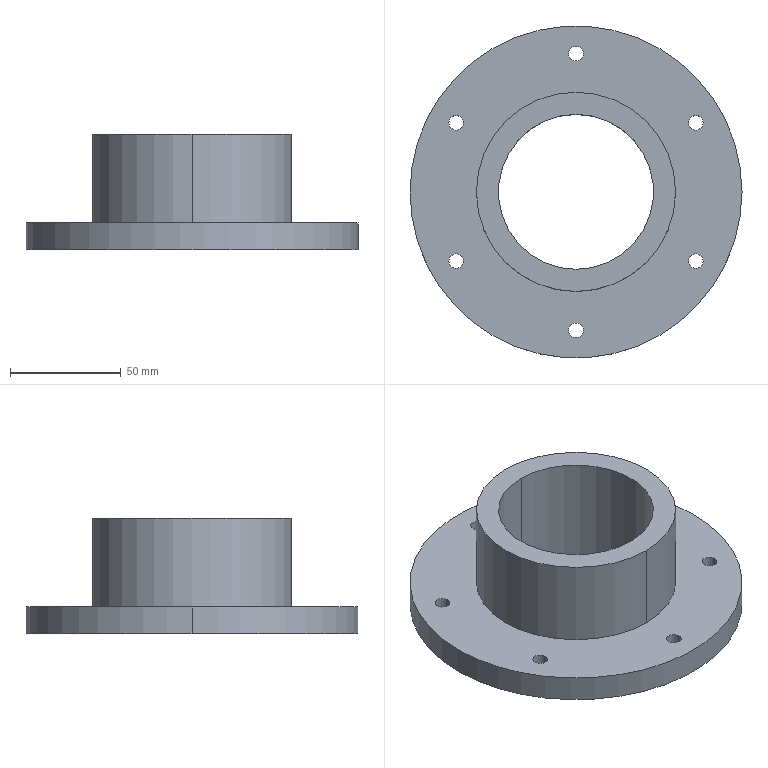Part | SolidWorks | features BaseBody 1 | 1 solid | 39 faces | box 150 x 150 x 52 mm | volume 261462 mm3 | cylinder 30 | plane 9 | commonest cylinder face diameters 6.6 x12 11 x12 70 x2 90 x2 150 x2
STEP:
#1=CARTESIAN_POINT('',(-54.127,36.75,6.8));
#2=VERTEX_POINT('',#1);
#3=CARTESIAN_POINT('',(-54.127,25.75,6.8));
#4=VERTEX_POINT('',#3);
#5=CARTESIAN_POINT('',(-54.127,31.25,6.8));
#6=DIRECTION('',(0.,0.,1.));
#7=DIRECTION('',(0.,1.,0.));
#8=AXIS2_PLACEMENT_3D('',#5,#6,#7);
#9=CIRCLE('',#8,5.5);
#10=EDGE_CURVE('',#2,#4,#9,.T.);
#11=ORIENTED_EDGE('',*,*,#10,.T.);
#12=CARTESIAN_POINT('',(-54.127,25.75,0.));
#13=VERTEX_POINT('',#12);
#14=CARTESIAN_POINT('',(-54.127,25.75,6.8));
#15=DIRECTION('',(0.,0.,-1.));
#16=VECTOR('',#15,1000.);
#17=LINE('',#14,#16);
#18=EDGE_CURVE('',#4,#13,#17,.T.);
#19=ORIENTED_EDGE('',*,*,#18,.T.);
#20=CARTESIAN_POINT('',(-54.127,36.75,0.));
#21=VERTEX_POINT('',#20);
#22=CARTESIAN_POINT('',(-54.127,31.25,0.));
#23=DIRECTION('',(0.,0.,-1.));
#24=DIRECTION('',(0.,1.,0.));
#25=AXIS2_PLACEMENT_3D('',#22,#23,#24);
#26=CIRCLE('',#25,5.5);
#27=EDGE_CURVE('',#13,#21,#26,.T.);
#28=ORIENTED_EDGE('',*,*,#27,.T.);
#29=CARTESIAN_POINT('',(-54.127,36.75,6.8));
#30=DIRECTION('',(0.,0.,-1.));
#31=VECTOR('',#30,1000.);
#32=LINE('',#29,#31);
#33=EDGE_CURVE('',#2,#21,#32,.T.);
#34=ORIENTED_EDGE('',*,*,#33,.F.);
#35=EDGE_LOOP('',(#11,#19,#28,#34));
#36=FACE_OUTER_BOUND('',#35,.T.);
#37=CARTESIAN_POINT('',(-54.127,31.25,6.8));
#38=DIRECTION('',(0.,0.,-1.));
#39=DIRECTION('',(0.,1.,0.));
#40=AXIS2_PLACEMENT_3D('',#37,#38,#39);
#41=CYLINDRICAL_SURFACE('',#40,5.5);
#42=ADVANCED_FACE('',(#36),#41,.F.);
#43=CARTESIAN_POINT('',(0.,35.,52.));
#44=VERTEX_POINT('',#43);
#45=CARTESIAN_POINT('',(0.,-35.,52.));
#46=VERTEX_POINT('',#45);
#47=CARTESIAN_POINT('',(0.,0.,52.));
#48=DIRECTION('',(0.,0.,1.));
#49=DIRECTION('',(0.,1.,0.));
#50=AXIS2_PLACEMENT_3D('',#47,#48,#49);
#51=CIRCLE('',#50,35.);
#52=EDGE_CURVE('',#44,#46,#51,.T.);
#53=ORIENTED_EDGE('',*,*,#52,.T.);
#54=CARTESIAN_POINT('',(0.,-35.,0.));
#55=VERTEX_POINT('',#54);
#56=CARTESIAN_POINT('',(0.,-35.,52.));
#57=DIRECTION('',(0.,0.,-1.));
#58=VECTOR('',#57,1000.);
#59=LINE('',#56,#58);
#60=EDGE_CURVE('',#46,#55,#59,.T.);
#61=ORIENTED_EDGE('',*,*,#60,.T.);
#62=CARTESIAN_POINT('',(0.,35.,0.));
#63=VERTEX_POINT('',#62);
#64=CARTESIAN_POINT('',(0.,0.,0.));
#65=DIRECTION('',(0.,0.,-1.));
#66=DIRECTION('',(0.,1.,0.));
#67=AXIS2_PLACEMENT_3D('',#64,#65,#66);
#68=CIRCLE('',#67,35.);
#69=EDGE_CURVE('',#55,#63,#68,.T.);
#70=ORIENTED_EDGE('',*,*,#69,.T.);
#71=CARTESIAN_POINT('',(0.,35.,52.));
#72=DIRECTION('',(0.,0.,-1.));
#73=VECTOR('',#72,1000.);
#74=LINE('',#71,#73);
#75=EDGE_CURVE('',#44,#63,#74,.T.);
#76=ORIENTED_EDGE('',*,*,#75,.F.);
#77=EDGE_LOOP('',(#53,#61,#70,#76));
#78=FACE_OUTER_BOUND('',#77,.T.);
#79=CARTESIAN_POINT('',(0.,0.,52.));
#80=DIRECTION('',(0.,0.,-1.));
#81=DIRECTION('',(0.,1.,0.));
#82=AXIS2_PLACEMENT_3D('',#79,#80,#81);
#83=CYLINDRICAL_SURFACE('',#82,35.);
#84=ADVANCED_FACE('',(#78),#83,.F.);
#85=CARTESIAN_POINT('',(0.,68.,6.8));
#86=VERTEX_POINT('',#85);
#87=CARTESIAN_POINT('',(0.,57.,6.8));
#88=VERTEX_POINT('',#87);
#89=CARTESIAN_POINT('',(0.,62.5,6.8));
#90=DIRECTION('',(0.,0.,1.));
#91=DIRECTION('',(0.,1.,0.));
#92=AXIS2_PLACEMENT_3D('',#89,#90,#91);
#93=CIRCLE('',#92,5.5);
#94=EDGE_CURVE('',#86,#88,#93,.T.);
#95=ORIENTED_EDGE('',*,*,#94,.T.);
#96=CARTESIAN_POINT('',(0.,57.,0.));
#97=VERTEX_POINT('',#96);
#98=CARTESIAN_POINT('',(0.,57.,6.8));
#99=DIRECTION('',(0.,0.,-1.));
#100=VECTOR('',#99,1000.);
#101=LINE('',#98,#100);
#102=EDGE_CURVE('',#88,#97,#101,.T.);
#103=ORIENTED_EDGE('',*,*,#102,.T.);
#104=CARTESIAN_POINT('',(0.,68.,0.));
#105=VERTEX_POINT('',#104);
#106=CARTESIAN_POINT('',(0.,62.5,0.));
#107=DIRECTION('',(0.,0.,-1.));
#108=DIRECTION('',(0.,1.,0.));
#109=AXIS2_PLACEMENT_3D('',#106,#107,#108);
#110=CIRCLE('',#109,5.5);
#111=EDGE_CURVE('',#97,#105,#110,.T.);
#112=ORIENTED_EDGE('',*,*,#111,.T.);
#113=CARTESIAN_POINT('',(0.,68.,6.8));
#114=DIRECTION('',(0.,0.,-1.));
#115=VECTOR('',#114,1000.);
#116=LINE('',#113,#115);
#117=EDGE_CURVE('',#86,#105,#116,.T.);
#118=ORIENTED_EDGE('',*,*,#117,.F.);
#119=EDGE_LOOP('',(#95,#103,#112,#118));
#120=FACE_OUTER_BOUND('',#119,.T.);
#121=CARTESIAN_POINT('',(0.,62.5,6.8));
#122=DIRECTION('',(0.,0.,-1.));
#123=DIRECTION('',(0.,1.,0.));
#124=AXIS2_PLACEMENT_3D('',#121,#122,#123);
#125=CYLINDRICAL_SURFACE('',#124,5.5);
#126=ADVANCED_FACE('',(#120),#125,.F.);
#127=CARTESIAN_POINT('',(54.127,36.75,6.8));
#128=VERTEX_POINT('',#127);
#129=CARTESIAN_POINT('',(54.127,25.75,6.8));
#130=VERTEX_POINT('',#129);
#131=CARTESIAN_POINT('',(54.127,31.25,6.8));
#132=DIRECTION('',(0.,0.,1.));
#133=DIRECTION('',(0.,1.,0.));
#134=AXIS2_PLACEMENT_3D('',#131,#132,#133);
#135=CIRCLE('',#134,5.5);
#136=EDGE_CURVE('',#128,#130,#135,.T.);
#137=ORIENTED_EDGE('',*,*,#136,.T.);
#138=CARTESIAN_POINT('',(54.127,25.75,0.));
#139=VERTEX_POINT('',#138);
#140=CARTESIAN_POINT('',(54.127,25.75,6.8));
#141=DIRECTION('',(0.,0.,-1.));
#142=VECTOR('',#141,1000.);
#143=LINE('',#140,#142);
#144=EDGE_CURVE('',#130,#139,#143,.T.);
#145=ORIENTED_EDGE('',*,*,#144,.T.);
#146=CARTESIAN_POINT('',(54.127,36.75,0.));
#147=VERTEX_POINT('',#146);
#148=CARTESIAN_POINT('',(54.127,31.25,0.));
#149=DIRECTION('',(0.,0.,-1.));
#150=DIRECTION('',(0.,1.,0.));
#151=AXIS2_PLACEMENT_3D('',#148,#149,#150);
#152=CIRCLE('',#151,5.5);
#153=EDGE_CURVE('',#139,#147,#152,.T.);
#154=ORIENTED_EDGE('',*,*,#153,.T.);
#155=CARTESIAN_POINT('',(54.127,36.75,6.8));
#156=DIRECTION('',(0.,0.,-1.));
#157=VECTOR('',#156,1000.);
#158=LINE('',#155,#157);
#159=EDGE_CURVE('',#128,#147,#158,.T.);
#160=ORIENTED_EDGE('',*,*,#159,.F.);
#161=EDGE_LOOP('',(#137,#145,#154,#160));
#162=FACE_OUTER_BOUND('',#161,.T.);
#163=CARTESIAN_POINT('',(54.127,31.25,6.8));
#164=DIRECTION('',(0.,0.,-1.));
#165=DIRECTION('',(0.,1.,0.));
#166=AXIS2_PLACEMENT_3D('',#163,#164,#165);
#167=CYLINDRICAL_SURFACE('',#166,5.5);
#168=ADVANCED_FACE('',(#162),#167,.F.);
#169=CARTESIAN_POINT('',(54.127,-25.75,6.8));
#170=VERTEX_POINT('',#169);
#171=CARTESIAN_POINT('',(54.127,-36.75,6.8));
#172=VERTEX_POINT('',#171);
#173=CARTESIAN_POINT('',(54.127,-31.25,6.8));
#174=DIRECTION('',(0.,0.,1.));
#175=DIRECTION('',(0.,1.,0.));
#176=AXIS2_PLACEMENT_3D('',#173,#174,#175);
#177=CIRCLE('',#176,5.5);
#178=EDGE_CURVE('',#170,#172,#177,.T.);
#179=ORIENTED_EDGE('',*,*,#178,.T.);
#180=CARTESIAN_POINT('',(54.127,-36.75,0.));
#181=VERTEX_POINT('',#180);
#182=CARTESIAN_POINT('',(54.127,-36.75,6.8));
#183=DIRECTION('',(0.,0.,-1.));
#184=VECTOR('',#183,1000.);
#185=LINE('',#182,#184);
#186=EDGE_CURVE('',#172,#181,#185,.T.);
#187=ORIENTED_EDGE('',*,*,#186,.T.);
#188=CARTESIAN_POINT('',(54.127,-25.75,0.));
#189=VERTEX_POINT('',#188);
#190=CARTESIAN_POINT('',(54.127,-31.25,0.));
#191=DIRECTION('',(0.,0.,-1.));
#192=DIRECTION('',(0.,1.,0.));
#193=AXIS2_PLACEMENT_3D('',#190,#191,#192);
#194=CIRCLE('',#193,5.5);
#195=EDGE_CURVE('',#181,#189,#194,.T.);
#196=ORIENTED_EDGE('',*,*,#195,.T.);
#197=CARTESIAN_POINT('',(54.127,-25.75,6.8));
#198=DIRECTION('',(0.,0.,-1.));
#199=VECTOR('',#198,1000.);
#200=LINE('',#197,#199);
#201=EDGE_CURVE('',#170,#189,#200,.T.);
#202=ORIENTED_EDGE('',*,*,#201,.F.);
#203=EDGE_LOOP('',(#179,#187,#196,#202));
#204=FACE_OUTER_BOUND('',#203,.T.);
#205=CARTESIAN_POINT('',(54.127,-31.25,6.8));
#206=DIRECTION('',(0.,0.,-1.));
#207=DIRECTION('',(0.,1.,0.));
#208=AXIS2_PLACEMENT_3D('',#205,#206,#207);
#209=CYLINDRICAL_SURFACE('',#208,5.5);
#210=ADVANCED_FACE('',(#204),#209,.F.);
#211=CARTESIAN_POINT('',(0.,-57.,6.8));
#212=VERTEX_POINT('',#211);
#213=CARTESIAN_POINT('',(0.,-68.,6.8));
#214=VERTEX_POINT('',#213);
#215=CARTESIAN_POINT('',(0.,-62.5,6.8));
#216=DIRECTION('',(0.,0.,1.));
#217=DIRECTION('',(0.,1.,0.));
#218=AXIS2_PLACEMENT_3D('',#215,#216,#217);
#219=CIRCLE('',#218,5.5);
#220=EDGE_CURVE('',#212,#214,#219,.T.);
#221=ORIENTED_EDGE('',*,*,#220,.T.);
#222=CARTESIAN_POINT('',(0.,-68.,0.));
#223=VERTEX_POINT('',#222);
#224=CARTESIAN_POINT('',(0.,-68.,6.8));
#225=DIRECTION('',(0.,0.,-1.));
#226=VECTOR('',#225,1000.);
#227=LINE('',#224,#226);
#228=EDGE_CURVE('',#214,#223,#227,.T.);
#229=ORIENTED_EDGE('',*,*,#228,.T.);
#230=CARTESIAN_POINT('',(0.,-57.,0.));
#231=VERTEX_POINT('',#230);
#232=CARTESIAN_POINT('',(0.,-62.5,0.));
#233=DIRECTION('',(0.,0.,-1.));
#234=DIRECTION('',(0.,1.,0.));
#235=AXIS2_PLACEMENT_3D('',#232,#233,#234);
#236=CIRCLE('',#235,5.5);
#237=EDGE_CURVE('',#223,#231,#236,.T.);
#238=ORIENTED_EDGE('',*,*,#237,.T.);
#239=CARTESIAN_POINT('',(0.,-57.,6.8));
#240=DIRECTION('',(0.,0.,-1.));
#241=VECTOR('',#240,1000.);
#242=LINE('',#239,#241);
#243=EDGE_CURVE('',#212,#231,#242,.T.);
#244=ORIENTED_EDGE('',*,*,#243,.F.);
#245=EDGE_LOOP('',(#221,#229,#238,#244));
#246=FACE_OUTER_BOUND('',#245,.T.);
#247=CARTESIAN_POINT('',(0.,-62.5,6.8));
#248=DIRECTION('',(0.,0.,-1.));
#249=DIRECTION('',(0.,1.,0.));
#250=AXIS2_PLACEMENT_3D('',#247,#248,#249);
#251=CYLINDRICAL_SURFACE('',#250,5.5);
#252=ADVANCED_FACE('',(#246),#251,.F.);
#253=CARTESIAN_POINT('',(-54.127,-25.75,6.8));
#254=VERTEX_POINT('',#253);
#255=CARTESIAN_POINT('',(-54.127,-36.75,6.8));
#256=VERTEX_POINT('',#255);
#257=CARTESIAN_POINT('',(-54.127,-31.25,6.8));
#258=DIRECTION('',(0.,0.,1.));
#259=DIRECTION('',(0.,1.,0.));
#260=AXIS2_PLACEMENT_3D('',#257,#258,#259);
#261=CIRCLE('',#260,5.5);
#262=EDGE_CURVE('',#254,#256,#261,.T.);
#263=ORIENTED_EDGE('',*,*,#262,.T.);
#264=CARTESIAN_POINT('',(-54.127,-36.75,0.));
#265=VERTEX_POINT('',#264);
#266=CARTESIAN_POINT('',(-54.127,-36.75,6.8));
#267=DIRECTION('',(0.,0.,-1.));
#268=VECTOR('',#267,1000.);
#269=LINE('',#266,#268);
#270=EDGE_CURVE('',#256,#265,#269,.T.);
#271=ORIENTED_EDGE('',*,*,#270,.T.);
#272=CARTESIAN_POINT('',(-54.127,-25.75,0.));
#273=VERTEX_POINT('',#272);
#274=CARTESIAN_POINT('',(-54.127,-31.25,0.));
#275=DIRECTION('',(0.,0.,-1.));
#276=DIRECTION('',(0.,1.,0.));
#277=AXIS2_PLACEMENT_3D('',#274,#275,#276);
#278=CIRCLE('',#277,5.5);
#279=EDGE_CURVE('',#265,#273,#278,.T.);
#280=ORIENTED_EDGE('',*,*,#279,.T.);
#281=CARTESIAN_POINT('',(-54.127,-25.75,6.8));
#282=DIRECTION('',(0.,0.,-1.));
#283=VECTOR('',#282,1000.);
#284=LINE('',#281,#283);
#285=EDGE_CURVE('',#254,#273,#284,.T.);
#286=ORIENTED_EDGE('',*,*,#285,.F.);
#287=EDGE_LOOP('',(#263,#271,#280,#286));
#288=FACE_OUTER_BOUND('',#287,.T.);
#289=CARTESIAN_POINT('',(-54.127,-31.25,6.8));
#290=DIRECTION('',(0.,0.,-1.));
#291=DIRECTION('',(0.,1.,0.));
#292=AXIS2_PLACEMENT_3D('',#289,#290,#291);
#293=CYLINDRICAL_SURFACE('',#292,5.5);
#294=ADVANCED_FACE('',(#288),#293,.F.);
#295=CARTESIAN_POINT('',(75.,0.,12.));
#296=VERTEX_POINT('',#295);
#297=CARTESIAN_POINT('',(-75.,0.,12.));
#298=VERTEX_POINT('',#297);
#299=CARTESIAN_POINT('',(0.,0.,12.));
#300=DIRECTION('',(0.,0.,1.));
#301=DIRECTION('',(-1.,0.,0.));
#302=AXIS2_PLACEMENT_3D('',#299,#300,#301);
#303=CIRCLE('',#302,75.);
#304=EDGE_CURVE('',#296,#298,#303,.T.);
#305=ORIENTED_EDGE('',*,*,#304,.F.);
#306=CARTESIAN_POINT('',(75.,0.,0.));
#307=VERTEX_POINT('',#306);
#308=CARTESIAN_POINT('',(75.,0.,12.));
#309=DIRECTION('',(0.,0.,-1.));
#310=VECTOR('',#309,1000.);
#311=LINE('',#308,#310);
#312=EDGE_CURVE('',#296,#307,#311,.T.);
#313=ORIENTED_EDGE('',*,*,#312,.T.);
#314=CARTESIAN_POINT('',(-75.,0.,0.));
#315=VERTEX_POINT('',#314);
#316=CARTESIAN_POINT('',(0.,0.,0.));
#317=DIRECTION('',(0.,0.,1.));
#318=DIRECTION('',(-1.,0.,0.));
#319=AXIS2_PLACEMENT_3D('',#316,#317,#318);
#320=CIRCLE('',#319,75.);
#321=EDGE_CURVE('',#307,#315,#320,.T.);
#322=ORIENTED_EDGE('',*,*,#321,.T.);
#323=CARTESIAN_POINT('',(-75.,0.,12.));
#324=DIRECTION('',(0.,0.,-1.));
#325=VECTOR('',#324,1000.);
#326=LINE('',#323,#325);
#327=EDGE_CURVE('',#298,#315,#326,.T.);
#328=ORIENTED_EDGE('',*,*,#327,.F.);
#329=EDGE_LOOP('',(#305,#313,#322,#328));
#330=FACE_OUTER_BOUND('',#329,.T.);
#331=CARTESIAN_POINT('',(0.,0.,12.));
#332=DIRECTION('',(0.,0.,-1.));
#333=DIRECTION('',(-1.,0.,0.));
#334=AXIS2_PLACEMENT_3D('',#331,#332,#333);
#335=CYLINDRICAL_SURFACE('',#334,75.);
#336=ADVANCED_FACE('',(#330),#335,.T.);
#337=CARTESIAN_POINT('',(-57.427,31.25,12.));
#338=VERTEX_POINT('',#337);
#339=CARTESIAN_POINT('',(-50.827,31.25,12.));
#340=VERTEX_POINT('',#339);
#341=CARTESIAN_POINT('',(-54.127,31.25,12.));
#342=DIRECTION('',(0.,0.,1.));
#343=DIRECTION('',(-1.,0.,0.));
#344=AXIS2_PLACEMENT_3D('',#341,#342,#343);
#345=CIRCLE('',#344,3.3);
#346=EDGE_CURVE('',#338,#340,#345,.T.);
#347=ORIENTED_EDGE('',*,*,#346,.T.);
#348=CARTESIAN_POINT('',(-50.827,31.25,6.8));
#349=VERTEX_POINT('',#348);
#350=CARTESIAN_POINT('',(-50.827,31.25,12.));
#351=DIRECTION('',(0.,0.,-1.));
#352=VECTOR('',#351,1000.);
#353=LINE('',#350,#352);
#354=EDGE_CURVE('',#340,#349,#353,.T.);
#355=ORIENTED_EDGE('',*,*,#354,.T.);
#356=CARTESIAN_POINT('',(-57.427,31.25,6.8));
#357=VERTEX_POINT('',#356);
#358=CARTESIAN_POINT('',(-54.127,31.25,6.8));
#359=DIRECTION('',(0.,0.,-1.));
#360=DIRECTION('',(-1.,0.,0.));
#361=AXIS2_PLACEMENT_3D('',#358,#359,#360);
#362=CIRCLE('',#361,3.3);
#363=EDGE_CURVE('',#349,#357,#362,.T.);
#364=ORIENTED_EDGE('',*,*,#363,.T.);
#365=CARTESIAN_POINT('',(-57.427,31.25,12.));
#366=DIRECTION('',(0.,0.,-1.));
#367=VECTOR('',#366,1000.);
#368=LINE('',#365,#367);
#369=EDGE_CURVE('',#338,#357,#368,.T.);
#370=ORIENTED_EDGE('',*,*,#369,.F.);
#371=EDGE_LOOP('',(#347,#355,#364,#370));
#372=FACE_OUTER_BOUND('',#371,.T.);
#373=CARTESIAN_POINT('',(-54.127,31.25,12.));
#374=DIRECTION('',(0.,0.,-1.));
#375=DIRECTION('',(-1.,0.,0.));
#376=AXIS2_PLACEMENT_3D('',#373,#374,#375);
#377=CYLINDRICAL_SURFACE('',#376,3.3);
#378=ADVANCED_FACE('',(#372),#377,.F.);
#379=CARTESIAN_POINT('',(0.,-45.,52.));
#380=VERTEX_POINT('',#379);
#381=CARTESIAN_POINT('',(0.,45.,52.));
#382=VERTEX_POINT('',#381);
#383=CARTESIAN_POINT('',(0.,0.,52.));
#384=DIRECTION('',(0.,0.,1.));
#385=DIRECTION('',(0.,1.,0.));
#386=AXIS2_PLACEMENT_3D('',#383,#384,#385);
#387=CIRCLE('',#386,45.);
#388=EDGE_CURVE('',#380,#382,#387,.T.);
#389=ORIENTED_EDGE('',*,*,#388,.F.);
#390=CARTESIAN_POINT('',(0.,-45.,12.));
#391=VERTEX_POINT('',#390);
#392=CARTESIAN_POINT('',(0.,-45.,52.));
#393=DIRECTION('',(0.,0.,-1.));
#394=VECTOR('',#393,1000.);
#395=LINE('',#392,#394);
#396=EDGE_CURVE('',#380,#391,#395,.T.);
#397=ORIENTED_EDGE('',*,*,#396,.T.);
#398=CARTESIAN_POINT('',(0.,45.,12.));
#399=VERTEX_POINT('',#398);
#400=CARTESIAN_POINT('',(0.,0.,12.));
#401=DIRECTION('',(0.,0.,-1.));
#402=DIRECTION('',(0.,1.,0.));
#403=AXIS2_PLACEMENT_3D('',#400,#401,#402);
#404=CIRCLE('',#403,45.);
#405=EDGE_CURVE('',#399,#391,#404,.T.);
#406=ORIENTED_EDGE('',*,*,#405,.F.);
#407=CARTESIAN_POINT('',(0.,45.,52.));
#408=DIRECTION('',(0.,0.,-1.));
#409=VECTOR('',#408,1000.);
#410=LINE('',#407,#409);
#411=EDGE_CURVE('',#382,#399,#410,.T.);
#412=ORIENTED_EDGE('',*,*,#411,.F.);
#413=EDGE_LOOP('',(#389,#397,#406,#412));
#414=FACE_OUTER_BOUND('',#413,.T.);
#415=CARTESIAN_POINT('',(0.,0.,52.));
#416=DIRECTION('',(0.,0.,-1.));
#417=DIRECTION('',(0.,1.,0.));
#418=AXIS2_PLACEMENT_3D('',#415,#416,#417);
#419=CYLINDRICAL_SURFACE('',#418,45.);
#420=ADVANCED_FACE('',(#414),#419,.T.);
#421=CARTESIAN_POINT('',(3.3,62.5,12.));
#422=VERTEX_POINT('',#421);
#423=CARTESIAN_POINT('',(-3.3,62.5,12.));
#424=VERTEX_POINT('',#423);
#425=CARTESIAN_POINT('',(0.,62.5,12.));
#426=DIRECTION('',(0.,0.,-1.));
#427=DIRECTION('',(-1.,0.,0.));
#428=AXIS2_PLACEMENT_3D('',#425,#426,#427);
#429=CIRCLE('',#428,3.3);
#430=EDGE_CURVE('',#422,#424,#429,.T.);
#431=ORIENTED_EDGE('',*,*,#430,.F.);
#432=CARTESIAN_POINT('',(3.3,62.5,6.8));
#433=VERTEX_POINT('',#432);
#434=CARTESIAN_POINT('',(3.3,62.5,12.));
#435=DIRECTION('',(0.,0.,-1.));
#436=VECTOR('',#435,1000.);
#437=LINE('',#434,#436);
#438=EDGE_CURVE('',#422,#433,#437,.T.);
#439=ORIENTED_EDGE('',*,*,#438,.T.);
#440=CARTESIAN_POINT('',(-3.3,62.5,6.8));
#441=VERTEX_POINT('',#440);
#442=CARTESIAN_POINT('',(0.,62.5,6.8));
#443=DIRECTION('',(0.,0.,-1.));
#444=DIRECTION('',(-1.,0.,0.));
#445=AXIS2_PLACEMENT_3D('',#442,#443,#444);
#446=CIRCLE('',#445,3.3);
#447=EDGE_CURVE('',#433,#441,#446,.T.);
#448=ORIENTED_EDGE('',*,*,#447,.T.);
#449=CARTESIAN_POINT('',(-3.3,62.5,12.));
#450=DIRECTION('',(0.,0.,-1.));
#451=VECTOR('',#450,1000.);
#452=LINE('',#449,#451);
#453=EDGE_CURVE('',#424,#441,#452,.T.);
#454=ORIENTED_EDGE('',*,*,#453,.F.);
#455=EDGE_LOOP('',(#431,#439,#448,#454));
#456=FACE_OUTER_BOUND('',#455,.T.);
#457=CARTESIAN_POINT('',(0.,62.5,12.));
#458=DIRECTION('',(0.,0.,-1.));
#459=DIRECTION('',(-1.,0.,0.));
#460=AXIS2_PLACEMENT_3D('',#457,#458,#459);
#461=CYLINDRICAL_SURFACE('',#460,3.3);
#462=ADVANCED_FACE('',(#456),#461,.F.);
#463=CARTESIAN_POINT('',(57.427,31.25,12.));
#464=VERTEX_POINT('',#463);
#465=CARTESIAN_POINT('',(50.827,31.25,12.));
#466=VERTEX_POINT('',#465);
#467=CARTESIAN_POINT('',(54.127,31.25,12.));
#468=DIRECTION('',(0.,0.,-1.));
#469=DIRECTION('',(-1.,0.,0.));
#470=AXIS2_PLACEMENT_3D('',#467,#468,#469);
#471=CIRCLE('',#470,3.3);
#472=EDGE_CURVE('',#464,#466,#471,.T.);
#473=ORIENTED_EDGE('',*,*,#472,.F.);
#474=CARTESIAN_POINT('',(57.427,31.25,6.8));
#475=VERTEX_POINT('',#474);
#476=CARTESIAN_POINT('',(57.427,31.25,12.));
#477=DIRECTION('',(0.,0.,-1.));
#478=VECTOR('',#477,1000.);
#479=LINE('',#476,#478);
#480=EDGE_CURVE('',#464,#475,#479,.T.);
#481=ORIENTED_EDGE('',*,*,#480,.T.);
#482=CARTESIAN_POINT('',(50.827,31.25,6.8));
#483=VERTEX_POINT('',#482);
#484=CARTESIAN_POINT('',(54.127,31.25,6.8));
#485=DIRECTION('',(0.,0.,-1.));
#486=DIRECTION('',(-1.,0.,0.));
#487=AXIS2_PLACEMENT_3D('',#484,#485,#486);
#488=CIRCLE('',#487,3.3);
#489=EDGE_CURVE('',#475,#483,#488,.T.);
#490=ORIENTED_EDGE('',*,*,#489,.T.);
#491=CARTESIAN_POINT('',(50.827,31.25,12.));
#492=DIRECTION('',(0.,0.,-1.));
#493=VECTOR('',#492,1000.);
#494=LINE('',#491,#493);
#495=EDGE_CURVE('',#466,#483,#494,.T.);
#496=ORIENTED_EDGE('',*,*,#495,.F.);
#497=EDGE_LOOP('',(#473,#481,#490,#496));
#498=FACE_OUTER_BOUND('',#497,.T.);
#499=CARTESIAN_POINT('',(54.127,31.25,12.));
#500=DIRECTION('',(0.,0.,-1.));
#501=DIRECTION('',(-1.,0.,0.));
#502=AXIS2_PLACEMENT_3D('',#499,#500,#501);
#503=CYLINDRICAL_SURFACE('',#502,3.3);
#504=ADVANCED_FACE('',(#498),#503,.F.);
#505=CARTESIAN_POINT('',(57.427,-31.25,12.));
#506=VERTEX_POINT('',#505);
#507=CARTESIAN_POINT('',(50.827,-31.25,12.));
#508=VERTEX_POINT('',#507);
#509=CARTESIAN_POINT('',(54.127,-31.25,12.));
#510=DIRECTION('',(0.,0.,-1.));
#511=DIRECTION('',(-1.,0.,0.));
#512=AXIS2_PLACEMENT_3D('',#509,#510,#511);
#513=CIRCLE('',#512,3.3);
#514=EDGE_CURVE('',#506,#508,#513,.T.);
#515=ORIENTED_EDGE('',*,*,#514,.F.);
#516=CARTESIAN_POINT('',(57.427,-31.25,6.8));
#517=VERTEX_POINT('',#516);
#518=CARTESIAN_POINT('',(57.427,-31.25,12.));
#519=DIRECTION('',(0.,0.,-1.));
#520=VECTOR('',#519,1000.);
#521=LINE('',#518,#520);
#522=EDGE_CURVE('',#506,#517,#521,.T.);
#523=ORIENTED_EDGE('',*,*,#522,.T.);
#524=CARTESIAN_POINT('',(50.827,-31.25,6.8));
#525=VERTEX_POINT('',#524);
#526=CARTESIAN_POINT('',(54.127,-31.25,6.8));
#527=DIRECTION('',(0.,0.,-1.));
#528=DIRECTION('',(-1.,0.,0.));
#529=AXIS2_PLACEMENT_3D('',#526,#527,#528);
#530=CIRCLE('',#529,3.3);
#531=EDGE_CURVE('',#517,#525,#530,.T.);
#532=ORIENTED_EDGE('',*,*,#531,.T.);
#533=CARTESIAN_POINT('',(50.827,-31.25,12.));
#534=DIRECTION('',(0.,0.,-1.));
#535=VECTOR('',#534,1000.);
#536=LINE('',#533,#535);
#537=EDGE_CURVE('',#508,#525,#536,.T.);
#538=ORIENTED_EDGE('',*,*,#537,.F.);
#539=EDGE_LOOP('',(#515,#523,#532,#538));
#540=FACE_OUTER_BOUND('',#539,.T.);
#541=CARTESIAN_POINT('',(54.127,-31.25,12.));
#542=DIRECTION('',(0.,0.,-1.));
#543=DIRECTION('',(-1.,0.,0.));
#544=AXIS2_PLACEMENT_3D('',#541,#542,#543);
#545=CYLINDRICAL_SURFACE('',#544,3.3);
#546=ADVANCED_FACE('',(#540),#545,.F.);
#547=CARTESIAN_POINT('',(3.3,-62.5,12.));
#548=VERTEX_POINT('',#547);
#549=CARTESIAN_POINT('',(-3.3,-62.5,12.));
#550=VERTEX_POINT('',#549);
#551=CARTESIAN_POINT('',(0.,-62.5,12.));
#552=DIRECTION('',(0.,0.,-1.));
#553=DIRECTION('',(-1.,0.,0.));
#554=AXIS2_PLACEMENT_3D('',#551,#552,#553);
#555=CIRCLE('',#554,3.3);
#556=EDGE_CURVE('',#548,#550,#555,.T.);
#557=ORIENTED_EDGE('',*,*,#556,.F.);
#558=CARTESIAN_POINT('',(3.3,-62.5,6.8));
#559=VERTEX_POINT('',#558);
#560=CARTESIAN_POINT('',(3.3,-62.5,12.));
#561=DIRECTION('',(0.,0.,-1.));
#562=VECTOR('',#561,1000.);
#563=LINE('',#560,#562);
#564=EDGE_CURVE('',#548,#559,#563,.T.);
#565=ORIENTED_EDGE('',*,*,#564,.T.);
#566=CARTESIAN_POINT('',(-3.3,-62.5,6.8));
#567=VERTEX_POINT('',#566);
#568=CARTESIAN_POINT('',(0.,-62.5,6.8));
#569=DIRECTION('',(0.,0.,-1.));
#570=DIRECTION('',(-1.,0.,0.));
#571=AXIS2_PLACEMENT_3D('',#568,#569,#570);
#572=CIRCLE('',#571,3.3);
#573=EDGE_CURVE('',#559,#567,#572,.T.);
#574=ORIENTED_EDGE('',*,*,#573,.T.);
#575=CARTESIAN_POINT('',(-3.3,-62.5,12.));
#576=DIRECTION('',(0.,0.,-1.));
#577=VECTOR('',#576,1000.);
#578=LINE('',#575,#577);
#579=EDGE_CURVE('',#550,#567,#578,.T.);
#580=ORIENTED_EDGE('',*,*,#579,.F.);
#581=EDGE_LOOP('',(#557,#565,#574,#580));
#582=FACE_OUTER_BOUND('',#581,.T.);
#583=CARTESIAN_POINT('',(0.,-62.5,12.));
#584=DIRECTION('',(0.,0.,-1.));
#585=DIRECTION('',(-1.,0.,0.));
#586=AXIS2_PLACEMENT_3D('',#583,#584,#585);
#587=CYLINDRICAL_SURFACE('',#586,3.3);
#588=ADVANCED_FACE('',(#582),#587,.F.);
#589=CARTESIAN_POINT('',(-50.827,-31.25,12.));
#590=VERTEX_POINT('',#589);
#591=CARTESIAN_POINT('',(-57.427,-31.25,12.));
#592=VERTEX_POINT('',#591);
#593=CARTESIAN_POINT('',(-54.127,-31.25,12.));
#594=DIRECTION('',(0.,0.,-1.));
#595=DIRECTION('',(-1.,0.,0.));
#596=AXIS2_PLACEMENT_3D('',#593,#594,#595);
#597=CIRCLE('',#596,3.3);
#598=EDGE_CURVE('',#590,#592,#597,.T.);
#599=ORIENTED_EDGE('',*,*,#598,.F.);
#600=CARTESIAN_POINT('',(-50.827,-31.25,6.8));
#601=VERTEX_POINT('',#600);
#602=CARTESIAN_POINT('',(-50.827,-31.25,12.));
#603=DIRECTION('',(0.,0.,-1.));
#604=VECTOR('',#603,1000.);
#605=LINE('',#602,#604);
#606=EDGE_CURVE('',#590,#601,#605,.T.);
#607=ORIENTED_EDGE('',*,*,#606,.T.);
#608=CARTESIAN_POINT('',(-57.427,-31.25,6.8));
#609=VERTEX_POINT('',#608);
#610=CARTESIAN_POINT('',(-54.127,-31.25,6.8));
#611=DIRECTION('',(0.,0.,-1.));
#612=DIRECTION('',(-1.,0.,0.));
#613=AXIS2_PLACEMENT_3D('',#610,#611,#612);
#614=CIRCLE('',#613,3.3);
#615=EDGE_CURVE('',#601,#609,#614,.T.);
#616=ORIENTED_EDGE('',*,*,#615,.T.);
#617=CARTESIAN_POINT('',(-57.427,-31.25,12.));
#618=DIRECTION('',(0.,0.,-1.));
#619=VECTOR('',#618,1000.);
#620=LINE('',#617,#619);
#621=EDGE_CURVE('',#592,#609,#620,.T.);
#622=ORIENTED_EDGE('',*,*,#621,.F.);
#623=EDGE_LOOP('',(#599,#607,#616,#622));
#624=FACE_OUTER_BOUND('',#623,.T.);
#625=CARTESIAN_POINT('',(-54.127,-31.25,12.));
#626=DIRECTION('',(0.,0.,-1.));
#627=DIRECTION('',(-1.,0.,0.));
#628=AXIS2_PLACEMENT_3D('',#625,#626,#627);
#629=CYLINDRICAL_SURFACE('',#628,3.3);
#630=ADVANCED_FACE('',(#624),#629,.F.);
#631=ORIENTED_EDGE('',*,*,#18,.F.);
#632=CARTESIAN_POINT('',(-54.127,31.25,6.8));
#633=DIRECTION('',(0.,0.,1.));
#634=DIRECTION('',(0.,1.,0.));
#635=AXIS2_PLACEMENT_3D('',#632,#633,#634);
#636=CIRCLE('',#635,5.5);
#637=EDGE_CURVE('',#4,#2,#636,.T.);
#638=ORIENTED_EDGE('',*,*,#637,.T.);
#639=ORIENTED_EDGE('',*,*,#33,.T.);
#640=CARTESIAN_POINT('',(-54.127,31.25,0.));
#641=DIRECTION('',(0.,0.,-1.));
#642=DIRECTION('',(0.,1.,0.));
#643=AXIS2_PLACEMENT_3D('',#640,#641,#642);
#644=CIRCLE('',#643,5.5);
#645=EDGE_CURVE('',#21,#13,#644,.T.);
#646=ORIENTED_EDGE('',*,*,#645,.T.);
#647=EDGE_LOOP('',(#631,#638,#639,#646));
#648=FACE_OUTER_BOUND('',#647,.T.);
#649=CARTESIAN_POINT('',(-54.127,31.25,6.8));
#650=DIRECTION('',(0.,0.,-1.));
#651=DIRECTION('',(0.,1.,0.));
#652=AXIS2_PLACEMENT_3D('',#649,#650,#651);
#653=CYLINDRICAL_SURFACE('',#652,5.5);
#654=ADVANCED_FACE('',(#648),#653,.F.);
#655=CARTESIAN_POINT('',(0.,0.,0.));
#656=DIRECTION('',(0.,0.,-1.));
#657=DIRECTION('',(0.,1.,0.));
#658=AXIS2_PLACEMENT_3D('',#655,#656,#657);
#659=CIRCLE('',#658,35.);
#660=EDGE_CURVE('',#63,#55,#659,.T.);
#661=ORIENTED_EDGE('',*,*,#660,.F.);
#662=ORIENTED_EDGE('',*,*,#69,.F.);
#663=EDGE_LOOP('',(#661,#662));
#664=FACE_BOUND('',#663,.T.);
#665=CARTESIAN_POINT('',(0.,62.5,0.));
#666=DIRECTION('',(0.,0.,-1.));
#667=DIRECTION('',(0.,1.,0.));
#668=AXIS2_PLACEMENT_3D('',#665,#666,#667);
#669=CIRCLE('',#668,5.5);
#670=EDGE_CURVE('',#105,#97,#669,.T.);
#671=ORIENTED_EDGE('',*,*,#670,.F.);
#672=ORIENTED_EDGE('',*,*,#111,.F.);
#673=EDGE_LOOP('',(#671,#672));
#674=FACE_BOUND('',#673,.T.);
#675=CARTESIAN_POINT('',(54.127,31.25,0.));
#676=DIRECTION('',(0.,0.,-1.));
#677=DIRECTION('',(0.,1.,0.));
#678=AXIS2_PLACEMENT_3D('',#675,#676,#677);
#679=CIRCLE('',#678,5.5);
#680=EDGE_CURVE('',#147,#139,#679,.T.);
#681=ORIENTED_EDGE('',*,*,#680,.F.);
#682=ORIENTED_EDGE('',*,*,#153,.F.);
#683=EDGE_LOOP('',(#681,#682));
#684=FACE_BOUND('',#683,.T.);
#685=CARTESIAN_POINT('',(54.127,-31.25,0.));
#686=DIRECTION('',(0.,0.,-1.));
#687=DIRECTION('',(0.,1.,0.));
#688=AXIS2_PLACEMENT_3D('',#685,#686,#687);
#689=CIRCLE('',#688,5.5);
#690=EDGE_CURVE('',#189,#181,#689,.T.);
#691=ORIENTED_EDGE('',*,*,#690,.F.);
#692=ORIENTED_EDGE('',*,*,#195,.F.);
#693=EDGE_LOOP('',(#691,#692));
#694=FACE_BOUND('',#693,.T.);
#695=CARTESIAN_POINT('',(0.,-62.5,0.));
#696=DIRECTION('',(0.,0.,-1.));
#697=DIRECTION('',(0.,1.,0.));
#698=AXIS2_PLACEMENT_3D('',#695,#696,#697);
#699=CIRCLE('',#698,5.5);
#700=EDGE_CURVE('',#231,#223,#699,.T.);
#701=ORIENTED_EDGE('',*,*,#700,.F.);
#702=ORIENTED_EDGE('',*,*,#237,.F.);
#703=EDGE_LOOP('',(#701,#702));
#704=FACE_BOUND('',#703,.T.);
#705=CARTESIAN_POINT('',(-54.127,-31.25,0.));
#706=DIRECTION('',(0.,0.,-1.));
#707=DIRECTION('',(0.,1.,0.));
#708=AXIS2_PLACEMENT_3D('',#705,#706,#707);
#709=CIRCLE('',#708,5.5);
#710=EDGE_CURVE('',#273,#265,#709,.T.);
#711=ORIENTED_EDGE('',*,*,#710,.F.);
#712=ORIENTED_EDGE('',*,*,#279,.F.);
#713=EDGE_LOOP('',(#711,#712));
#714=FACE_BOUND('',#713,.T.);
#715=ORIENTED_EDGE('',*,*,#645,.F.);
#716=ORIENTED_EDGE('',*,*,#27,.F.);
#717=EDGE_LOOP('',(#715,#716));
#718=FACE_BOUND('',#717,.T.);
#719=CARTESIAN_POINT('',(0.,0.,0.));
#720=DIRECTION('',(0.,0.,1.));
#721=DIRECTION('',(-1.,0.,0.));
#722=AXIS2_PLACEMENT_3D('',#719,#720,#721);
#723=CIRCLE('',#722,75.);
#724=EDGE_CURVE('',#315,#307,#723,.T.);
#725=ORIENTED_EDGE('',*,*,#724,.F.);
#726=ORIENTED_EDGE('',*,*,#321,.F.);
#727=EDGE_LOOP('',(#725,#726));
#728=FACE_OUTER_BOUND('',#727,.T.);
#729=CARTESIAN_POINT('',(-75.9,-75.9,0.));
#730=DIRECTION('',(0.,0.,1.));
#731=DIRECTION('',(1.,0.,0.));
#732=AXIS2_PLACEMENT_3D('',#729,#730,#731);
#733=PLANE('',#732);
#734=ADVANCED_FACE('',(#664,#674,#684,#694,#704,#714,#718,#728),#733,.F.);
#735=CARTESIAN_POINT('',(-54.127,31.25,6.8));
#736=DIRECTION('',(0.,0.,-1.));
#737=DIRECTION('',(-1.,0.,0.));
#738=AXIS2_PLACEMENT_3D('',#735,#736,#737);
#739=CIRCLE('',#738,3.3);
#740=EDGE_CURVE('',#357,#349,#739,.T.);
#741=ORIENTED_EDGE('',*,*,#740,.F.);
#742=ORIENTED_EDGE('',*,*,#363,.F.);
#743=EDGE_LOOP('',(#741,#742));
#744=FACE_BOUND('',#743,.T.);
#745=ORIENTED_EDGE('',*,*,#10,.F.);
#746=ORIENTED_EDGE('',*,*,#637,.F.);
#747=EDGE_LOOP('',(#745,#746));
#748=FACE_OUTER_BOUND('',#747,.T.);
#749=CARTESIAN_POINT('',(-59.693,25.684,6.8));
#750=DIRECTION('',(0.,0.,1.));
#751=DIRECTION('',(1.,0.,0.));
#752=AXIS2_PLACEMENT_3D('',#749,#750,#751);
#753=PLANE('',#752);
#754=ADVANCED_FACE('',(#744,#748),#753,.F.);
#755=ORIENTED_EDGE('',*,*,#60,.F.);
#756=CARTESIAN_POINT('',(0.,0.,52.));
#757=DIRECTION('',(0.,0.,1.));
#758=DIRECTION('',(0.,1.,0.));
#759=AXIS2_PLACEMENT_3D('',#756,#757,#758);
#760=CIRCLE('',#759,35.);
#761=EDGE_CURVE('',#46,#44,#760,.T.);
#762=ORIENTED_EDGE('',*,*,#761,.T.);
#763=ORIENTED_EDGE('',*,*,#75,.T.);
#764=ORIENTED_EDGE('',*,*,#660,.T.);
#765=EDGE_LOOP('',(#755,#762,#763,#764));
#766=FACE_OUTER_BOUND('',#765,.T.);
#767=CARTESIAN_POINT('',(0.,0.,52.));
#768=DIRECTION('',(0.,0.,-1.));
#769=DIRECTION('',(0.,1.,0.));
#770=AXIS2_PLACEMENT_3D('',#767,#768,#769);
#771=CYLINDRICAL_SURFACE('',#770,35.);
#772=ADVANCED_FACE('',(#766),#771,.F.);
#773=ORIENTED_EDGE('',*,*,#102,.F.);
#774=CARTESIAN_POINT('',(0.,62.5,6.8));
#775=DIRECTION('',(0.,0.,1.));
#776=DIRECTION('',(0.,1.,0.));
#777=AXIS2_PLACEMENT_3D('',#774,#775,#776);
#778=CIRCLE('',#777,5.5);
#779=EDGE_CURVE('',#88,#86,#778,.T.);
#780=ORIENTED_EDGE('',*,*,#779,.T.);
#781=ORIENTED_EDGE('',*,*,#117,.T.);
#782=ORIENTED_EDGE('',*,*,#670,.T.);
#783=EDGE_LOOP('',(#773,#780,#781,#782));
#784=FACE_OUTER_BOUND('',#783,.T.);
#785=CARTESIAN_POINT('',(0.,62.5,6.8));
#786=DIRECTION('',(0.,0.,-1.));
#787=DIRECTION('',(0.,1.,0.));
#788=AXIS2_PLACEMENT_3D('',#785,#786,#787);
#789=CYLINDRICAL_SURFACE('',#788,5.5);
#790=ADVANCED_FACE('',(#784),#789,.F.);
#791=ORIENTED_EDGE('',*,*,#144,.F.);
#792=CARTESIAN_POINT('',(54.127,31.25,6.8));
#793=DIRECTION('',(0.,0.,1.));
#794=DIRECTION('',(0.,1.,0.));
#795=AXIS2_PLACEMENT_3D('',#792,#793,#794);
#796=CIRCLE('',#795,5.5);
#797=EDGE_CURVE('',#130,#128,#796,.T.);
#798=ORIENTED_EDGE('',*,*,#797,.T.);
#799=ORIENTED_EDGE('',*,*,#159,.T.);
#800=ORIENTED_EDGE('',*,*,#680,.T.);
#801=EDGE_LOOP('',(#791,#798,#799,#800));
#802=FACE_OUTER_BOUND('',#801,.T.);
#803=CARTESIAN_POINT('',(54.127,31.25,6.8));
#804=DIRECTION('',(0.,0.,-1.));
#805=DIRECTION('',(0.,1.,0.));
#806=AXIS2_PLACEMENT_3D('',#803,#804,#805);
#807=CYLINDRICAL_SURFACE('',#806,5.5);
#808=ADVANCED_FACE('',(#802),#807,.F.);
#809=ORIENTED_EDGE('',*,*,#186,.F.);
#810=CARTESIAN_POINT('',(54.127,-31.25,6.8));
#811=DIRECTION('',(0.,0.,1.));
#812=DIRECTION('',(0.,1.,0.));
#813=AXIS2_PLACEMENT_3D('',#810,#811,#812);
#814=CIRCLE('',#813,5.5);
#815=EDGE_CURVE('',#172,#170,#814,.T.);
#816=ORIENTED_EDGE('',*,*,#815,.T.);
#817=ORIENTED_EDGE('',*,*,#201,.T.);
#818=ORIENTED_EDGE('',*,*,#690,.T.);
#819=EDGE_LOOP('',(#809,#816,#817,#818));
#820=FACE_OUTER_BOUND('',#819,.T.);
#821=CARTESIAN_POINT('',(54.127,-31.25,6.8));
#822=DIRECTION('',(0.,0.,-1.));
#823=DIRECTION('',(0.,1.,0.));
#824=AXIS2_PLACEMENT_3D('',#821,#822,#823);
#825=CYLINDRICAL_SURFACE('',#824,5.5);
#826=ADVANCED_FACE('',(#820),#825,.F.);
#827=ORIENTED_EDGE('',*,*,#228,.F.);
#828=CARTESIAN_POINT('',(0.,-62.5,6.8));
#829=DIRECTION('',(0.,0.,1.));
#830=DIRECTION('',(0.,1.,0.));
#831=AXIS2_PLACEMENT_3D('',#828,#829,#830);
#832=CIRCLE('',#831,5.5);
#833=EDGE_CURVE('',#214,#212,#832,.T.);
#834=ORIENTED_EDGE('',*,*,#833,.T.);
#835=ORIENTED_EDGE('',*,*,#243,.T.);
#836=ORIENTED_EDGE('',*,*,#700,.T.);
#837=EDGE_LOOP('',(#827,#834,#835,#836));
#838=FACE_OUTER_BOUND('',#837,.T.);
#839=CARTESIAN_POINT('',(0.,-62.5,6.8));
#840=DIRECTION('',(0.,0.,-1.));
#841=DIRECTION('',(0.,1.,0.));
#842=AXIS2_PLACEMENT_3D('',#839,#840,#841);
#843=CYLINDRICAL_SURFACE('',#842,5.5);
#844=ADVANCED_FACE('',(#838),#843,.F.);
#845=ORIENTED_EDGE('',*,*,#270,.F.);
#846=CARTESIAN_POINT('',(-54.127,-31.25,6.8));
#847=DIRECTION('',(0.,0.,1.));
#848=DIRECTION('',(0.,1.,0.));
#849=AXIS2_PLACEMENT_3D('',#846,#847,#848);
#850=CIRCLE('',#849,5.5);
#851=EDGE_CURVE('',#256,#254,#850,.T.);
#852=ORIENTED_EDGE('',*,*,#851,.T.);
#853=ORIENTED_EDGE('',*,*,#285,.T.);
#854=ORIENTED_EDGE('',*,*,#710,.T.);
#855=EDGE_LOOP('',(#845,#852,#853,#854));
#856=FACE_OUTER_BOUND('',#855,.T.);
#857=CARTESIAN_POINT('',(-54.127,-31.25,6.8));
#858=DIRECTION('',(0.,0.,-1.));
#859=DIRECTION('',(0.,1.,0.));
#860=AXIS2_PLACEMENT_3D('',#857,#858,#859);
#861=CYLINDRICAL_SURFACE('',#860,5.5);
#862=ADVANCED_FACE('',(#856),#861,.F.);
#863=ORIENTED_EDGE('',*,*,#312,.F.);
#864=CARTESIAN_POINT('',(0.,0.,12.));
#865=DIRECTION('',(0.,0.,1.));
#866=DIRECTION('',(-1.,0.,0.));
#867=AXIS2_PLACEMENT_3D('',#864,#865,#866);
#868=CIRCLE('',#867,75.);
#869=EDGE_CURVE('',#298,#296,#868,.T.);
#870=ORIENTED_EDGE('',*,*,#869,.F.);
#871=ORIENTED_EDGE('',*,*,#327,.T.);
#872=ORIENTED_EDGE('',*,*,#724,.T.);
#873=EDGE_LOOP('',(#863,#870,#871,#872));
#874=FACE_OUTER_BOUND('',#873,.T.);
#875=CARTESIAN_POINT('',(0.,0.,12.));
#876=DIRECTION('',(0.,0.,-1.));
#877=DIRECTION('',(-1.,0.,0.));
#878=AXIS2_PLACEMENT_3D('',#875,#876,#877);
#879=CYLINDRICAL_SURFACE('',#878,75.);
#880=ADVANCED_FACE('',(#874),#879,.T.);
#881=ORIENTED_EDGE('',*,*,#354,.F.);
#882=CARTESIAN_POINT('',(-54.127,31.25,12.));
#883=DIRECTION('',(0.,0.,1.));
#884=DIRECTION('',(-1.,0.,0.));
#885=AXIS2_PLACEMENT_3D('',#882,#883,#884);
#886=CIRCLE('',#885,3.3);
#887=EDGE_CURVE('',#340,#338,#886,.T.);
#888=ORIENTED_EDGE('',*,*,#887,.T.);
#889=ORIENTED_EDGE('',*,*,#369,.T.);
#890=ORIENTED_EDGE('',*,*,#740,.T.);
#891=EDGE_LOOP('',(#881,#888,#889,#890));
#892=FACE_OUTER_BOUND('',#891,.T.);
#893=CARTESIAN_POINT('',(-54.127,31.25,12.));
#894=DIRECTION('',(0.,0.,-1.));
#895=DIRECTION('',(-1.,0.,0.));
#896=AXIS2_PLACEMENT_3D('',#893,#894,#895);
#897=CYLINDRICAL_SURFACE('',#896,3.3);
#898=ADVANCED_FACE('',(#892),#897,.F.);
#899=ORIENTED_EDGE('',*,*,#52,.F.);
#900=ORIENTED_EDGE('',*,*,#761,.F.);
#901=EDGE_LOOP('',(#899,#900));
#902=FACE_BOUND('',#901,.T.);
#903=CARTESIAN_POINT('',(0.,0.,52.));
#904=DIRECTION('',(0.,0.,1.));
#905=DIRECTION('',(0.,1.,0.));
#906=AXIS2_PLACEMENT_3D('',#903,#904,#905);
#907=CIRCLE('',#906,45.);
#908=EDGE_CURVE('',#382,#380,#907,.T.);
#909=ORIENTED_EDGE('',*,*,#908,.T.);
#910=ORIENTED_EDGE('',*,*,#388,.T.);
#911=EDGE_LOOP('',(#909,#910));
#912=FACE_OUTER_BOUND('',#911,.T.);
#913=CARTESIAN_POINT('',(-45.54,-45.54,52.));
#914=DIRECTION('',(0.,0.,1.));
#915=DIRECTION('',(1.,0.,0.));
#916=AXIS2_PLACEMENT_3D('',#913,#914,#915);
#917=PLANE('',#916);
#918=ADVANCED_FACE('',(#902,#912),#917,.T.);
#919=CARTESIAN_POINT('',(0.,62.5,6.8));
#920=DIRECTION('',(0.,0.,-1.));
#921=DIRECTION('',(-1.,0.,0.));
#922=AXIS2_PLACEMENT_3D('',#919,#920,#921);
#923=CIRCLE('',#922,3.3);
#924=EDGE_CURVE('',#441,#433,#923,.T.);
#925=ORIENTED_EDGE('',*,*,#924,.F.);
#926=ORIENTED_EDGE('',*,*,#447,.F.);
#927=EDGE_LOOP('',(#925,#926));
#928=FACE_BOUND('',#927,.T.);
#929=ORIENTED_EDGE('',*,*,#94,.F.);
#930=ORIENTED_EDGE('',*,*,#779,.F.);
#931=EDGE_LOOP('',(#929,#930));
#932=FACE_OUTER_BOUND('',#931,.T.);
#933=CARTESIAN_POINT('',(-5.566,56.934,6.8));
#934=DIRECTION('',(0.,0.,1.));
#935=DIRECTION('',(1.,0.,0.));
#936=AXIS2_PLACEMENT_3D('',#933,#934,#935);
#937=PLANE('',#936);
#938=ADVANCED_FACE('',(#928,#932),#937,.F.);
#939=CARTESIAN_POINT('',(54.127,31.25,6.8));
#940=DIRECTION('',(0.,0.,-1.));
#941=DIRECTION('',(-1.,0.,0.));
#942=AXIS2_PLACEMENT_3D('',#939,#940,#941);
#943=CIRCLE('',#942,3.3);
#944=EDGE_CURVE('',#483,#475,#943,.T.);
#945=ORIENTED_EDGE('',*,*,#944,.F.);
#946=ORIENTED_EDGE('',*,*,#489,.F.);
#947=EDGE_LOOP('',(#945,#946));
#948=FACE_BOUND('',#947,.T.);
#949=ORIENTED_EDGE('',*,*,#136,.F.);
#950=ORIENTED_EDGE('',*,*,#797,.F.);
#951=EDGE_LOOP('',(#949,#950));
#952=FACE_OUTER_BOUND('',#951,.T.);
#953=CARTESIAN_POINT('',(48.561,25.684,6.8));
#954=DIRECTION('',(0.,0.,1.));
#955=DIRECTION('',(1.,0.,0.));
#956=AXIS2_PLACEMENT_3D('',#953,#954,#955);
#957=PLANE('',#956);
#958=ADVANCED_FACE('',(#948,#952),#957,.F.);
#959=CARTESIAN_POINT('',(54.127,-31.25,6.8));
#960=DIRECTION('',(0.,0.,-1.));
#961=DIRECTION('',(-1.,0.,0.));
#962=AXIS2_PLACEMENT_3D('',#959,#960,#961);
#963=CIRCLE('',#962,3.3);
#964=EDGE_CURVE('',#525,#517,#963,.T.);
#965=ORIENTED_EDGE('',*,*,#964,.F.);
#966=ORIENTED_EDGE('',*,*,#531,.F.);
#967=EDGE_LOOP('',(#965,#966));
#968=FACE_BOUND('',#967,.T.);
#969=ORIENTED_EDGE('',*,*,#178,.F.);
#970=ORIENTED_EDGE('',*,*,#815,.F.);
#971=EDGE_LOOP('',(#969,#970));
#972=FACE_OUTER_BOUND('',#971,.T.);
#973=CARTESIAN_POINT('',(48.561,-36.816,6.8));
#974=DIRECTION('',(0.,0.,1.));
#975=DIRECTION('',(1.,0.,0.));
#976=AXIS2_PLACEMENT_3D('',#973,#974,#975);
#977=PLANE('',#976);
#978=ADVANCED_FACE('',(#968,#972),#977,.F.);
#979=CARTESIAN_POINT('',(0.,-62.5,6.8));
#980=DIRECTION('',(0.,0.,-1.));
#981=DIRECTION('',(-1.,0.,0.));
#982=AXIS2_PLACEMENT_3D('',#979,#980,#981);
#983=CIRCLE('',#982,3.3);
#984=EDGE_CURVE('',#567,#559,#983,.T.);
#985=ORIENTED_EDGE('',*,*,#984,.F.);
#986=ORIENTED_EDGE('',*,*,#573,.F.);
#987=EDGE_LOOP('',(#985,#986));
#988=FACE_BOUND('',#987,.T.);
#989=ORIENTED_EDGE('',*,*,#220,.F.);
#990=ORIENTED_EDGE('',*,*,#833,.F.);
#991=EDGE_LOOP('',(#989,#990));
#992=FACE_OUTER_BOUND('',#991,.T.);
#993=CARTESIAN_POINT('',(-5.566,-68.066,6.8));
#994=DIRECTION('',(0.,0.,1.));
#995=DIRECTION('',(1.,0.,0.));
#996=AXIS2_PLACEMENT_3D('',#993,#994,#995);
#997=PLANE('',#996);
#998=ADVANCED_FACE('',(#988,#992),#997,.F.);
#999=CARTESIAN_POINT('',(-54.127,-31.25,6.8));
#1000=DIRECTION('',(0.,0.,-1.));
#1001=DIRECTION('',(-1.,0.,0.));
#1002=AXIS2_PLACEMENT_3D('',#999,#1000,#1001);
#1003=CIRCLE('',#1002,3.3);
#1004=EDGE_CURVE('',#609,#601,#1003,.T.);
#1005=ORIENTED_EDGE('',*,*,#1004,.F.);
#1006=ORIENTED_EDGE('',*,*,#615,.F.);
#1007=EDGE_LOOP('',(#1005,#1006));
#1008=FACE_BOUND('',#1007,.T.);
#1009=ORIENTED_EDGE('',*,*,#262,.F.);
#1010=ORIENTED_EDGE('',*,*,#851,.F.);
#1011=EDGE_LOOP('',(#1009,#1010));
#1012=FACE_OUTER_BOUND('',#1011,.T.);
#1013=CARTESIAN_POINT('',(-59.693,-36.816,6.8));
#1014=DIRECTION('',(0.,0.,1.));
#1015=DIRECTION('',(1.,0.,0.));
#1016=AXIS2_PLACEMENT_3D('',#1013,#1014,#1015);
#1017=PLANE('',#1016);
#1018=ADVANCED_FACE('',(#1008,#1012),#1017,.F.);
#1019=ORIENTED_EDGE('',*,*,#405,.T.);
#1020=CARTESIAN_POINT('',(0.,0.,12.));
#1021=DIRECTION('',(0.,0.,-1.));
#1022=DIRECTION('',(0.,1.,0.));
#1023=AXIS2_PLACEMENT_3D('',#1020,#1021,#1022);
#1024=CIRCLE('',#1023,45.);
#1025=EDGE_CURVE('',#391,#399,#1024,.T.);
#1026=ORIENTED_EDGE('',*,*,#1025,.T.);
#1027=EDGE_LOOP('',(#1019,#1026));
#1028=FACE_BOUND('',#1027,.T.);
#1029=CARTESIAN_POINT('',(0.,62.5,12.));
#1030=DIRECTION('',(0.,0.,-1.));
#1031=DIRECTION('',(-1.,0.,0.));
#1032=AXIS2_PLACEMENT_3D('',#1029,#1030,#1031);
#1033=CIRCLE('',#1032,3.3);
#1034=EDGE_CURVE('',#424,#422,#1033,.T.);
#1035=ORIENTED_EDGE('',*,*,#1034,.T.);
#1036=ORIENTED_EDGE('',*,*,#430,.T.);
#1037=EDGE_LOOP('',(#1035,#1036));
#1038=FACE_BOUND('',#1037,.T.);
#1039=CARTESIAN_POINT('',(54.127,31.25,12.));
#1040=DIRECTION('',(0.,0.,-1.));
#1041=DIRECTION('',(-1.,0.,0.));
#1042=AXIS2_PLACEMENT_3D('',#1039,#1040,#1041);
#1043=CIRCLE('',#1042,3.3);
#1044=EDGE_CURVE('',#466,#464,#1043,.T.);
#1045=ORIENTED_EDGE('',*,*,#1044,.T.);
#1046=ORIENTED_EDGE('',*,*,#472,.T.);
#1047=EDGE_LOOP('',(#1045,#1046));
#1048=FACE_BOUND('',#1047,.T.);
#1049=CARTESIAN_POINT('',(54.127,-31.25,12.));
#1050=DIRECTION('',(0.,0.,-1.));
#1051=DIRECTION('',(-1.,0.,0.));
#1052=AXIS2_PLACEMENT_3D('',#1049,#1050,#1051);
#1053=CIRCLE('',#1052,3.3);
#1054=EDGE_CURVE('',#508,#506,#1053,.T.);
#1055=ORIENTED_EDGE('',*,*,#1054,.T.);
#1056=ORIENTED_EDGE('',*,*,#514,.T.);
#1057=EDGE_LOOP('',(#1055,#1056));
#1058=FACE_BOUND('',#1057,.T.);
#1059=CARTESIAN_POINT('',(0.,-62.5,12.));
#1060=DIRECTION('',(0.,0.,-1.));
#1061=DIRECTION('',(-1.,0.,0.));
#1062=AXIS2_PLACEMENT_3D('',#1059,#1060,#1061);
#1063=CIRCLE('',#1062,3.3);
#1064=EDGE_CURVE('',#550,#548,#1063,.T.);
#1065=ORIENTED_EDGE('',*,*,#1064,.T.);
#1066=ORIENTED_EDGE('',*,*,#556,.T.);
#1067=EDGE_LOOP('',(#1065,#1066));
#1068=FACE_BOUND('',#1067,.T.);
#1069=CARTESIAN_POINT('',(-54.127,-31.25,12.));
#1070=DIRECTION('',(0.,0.,-1.));
#1071=DIRECTION('',(-1.,0.,0.));
#1072=AXIS2_PLACEMENT_3D('',#1069,#1070,#1071);
#1073=CIRCLE('',#1072,3.3);
#1074=EDGE_CURVE('',#592,#590,#1073,.T.);
#1075=ORIENTED_EDGE('',*,*,#1074,.T.);
#1076=ORIENTED_EDGE('',*,*,#598,.T.);
#1077=EDGE_LOOP('',(#1075,#1076));
#1078=FACE_BOUND('',#1077,.T.);
#1079=ORIENTED_EDGE('',*,*,#346,.F.);
#1080=ORIENTED_EDGE('',*,*,#887,.F.);
#1081=EDGE_LOOP('',(#1079,#1080));
#1082=FACE_BOUND('',#1081,.T.);
#1083=ORIENTED_EDGE('',*,*,#869,.T.);
#1084=ORIENTED_EDGE('',*,*,#304,.T.);
#1085=EDGE_LOOP('',(#1083,#1084));
#1086=FACE_OUTER_BOUND('',#1085,.T.);
#1087=CARTESIAN_POINT('',(-75.9,-75.9,12.));
#1088=DIRECTION('',(0.,0.,1.));
#1089=DIRECTION('',(1.,0.,0.));
#1090=AXIS2_PLACEMENT_3D('',#1087,#1088,#1089);
#1091=PLANE('',#1090);
#1092=ADVANCED_FACE('',(#1028,#1038,#1048,#1058,#1068,#1078,#1082,#1086),#1091,.T.);
#1093=ORIENTED_EDGE('',*,*,#396,.F.);
#1094=ORIENTED_EDGE('',*,*,#908,.F.);
#1095=ORIENTED_EDGE('',*,*,#411,.T.);
#1096=ORIENTED_EDGE('',*,*,#1025,.F.);
#1097=EDGE_LOOP('',(#1093,#1094,#1095,#1096));
#1098=FACE_OUTER_BOUND('',#1097,.T.);
#1099=CARTESIAN_POINT('',(0.,0.,52.));
#1100=DIRECTION('',(0.,0.,-1.));
#1101=DIRECTION('',(0.,1.,0.));
#1102=AXIS2_PLACEMENT_3D('',#1099,#1100,#1101);
#1103=CYLINDRICAL_SURFACE('',#1102,45.);
#1104=ADVANCED_FACE('',(#1098),#1103,.T.);
#1105=ORIENTED_EDGE('',*,*,#438,.F.);
#1106=ORIENTED_EDGE('',*,*,#1034,.F.);
#1107=ORIENTED_EDGE('',*,*,#453,.T.);
#1108=ORIENTED_EDGE('',*,*,#924,.T.);
#1109=EDGE_LOOP('',(#1105,#1106,#1107,#1108));
#1110=FACE_OUTER_BOUND('',#1109,.T.);
#1111=CARTESIAN_POINT('',(0.,62.5,12.));
#1112=DIRECTION('',(0.,0.,-1.));
#1113=DIRECTION('',(-1.,0.,0.));
#1114=AXIS2_PLACEMENT_3D('',#1111,#1112,#1113);
#1115=CYLINDRICAL_SURFACE('',#1114,3.3);
#1116=ADVANCED_FACE('',(#1110),#1115,.F.);
#1117=ORIENTED_EDGE('',*,*,#480,.F.);
#1118=ORIENTED_EDGE('',*,*,#1044,.F.);
#1119=ORIENTED_EDGE('',*,*,#495,.T.);
#1120=ORIENTED_EDGE('',*,*,#944,.T.);
#1121=EDGE_LOOP('',(#1117,#1118,#1119,#1120));
#1122=FACE_OUTER_BOUND('',#1121,.T.);
#1123=CARTESIAN_POINT('',(54.127,31.25,12.));
#1124=DIRECTION('',(0.,0.,-1.));
#1125=DIRECTION('',(-1.,0.,0.));
#1126=AXIS2_PLACEMENT_3D('',#1123,#1124,#1125);
#1127=CYLINDRICAL_SURFACE('',#1126,3.3);
#1128=ADVANCED_FACE('',(#1122),#1127,.F.);
#1129=ORIENTED_EDGE('',*,*,#522,.F.);
#1130=ORIENTED_EDGE('',*,*,#1054,.F.);
#1131=ORIENTED_EDGE('',*,*,#537,.T.);
#1132=ORIENTED_EDGE('',*,*,#964,.T.);
#1133=EDGE_LOOP('',(#1129,#1130,#1131,#1132));
#1134=FACE_OUTER_BOUND('',#1133,.T.);
#1135=CARTESIAN_POINT('',(54.127,-31.25,12.));
#1136=DIRECTION('',(0.,0.,-1.));
#1137=DIRECTION('',(-1.,0.,0.));
#1138=AXIS2_PLACEMENT_3D('',#1135,#1136,#1137);
#1139=CYLINDRICAL_SURFACE('',#1138,3.3);
#1140=ADVANCED_FACE('',(#1134),#1139,.F.);
#1141=ORIENTED_EDGE('',*,*,#564,.F.);
#1142=ORIENTED_EDGE('',*,*,#1064,.F.);
#1143=ORIENTED_EDGE('',*,*,#579,.T.);
#1144=ORIENTED_EDGE('',*,*,#984,.T.);
#1145=EDGE_LOOP('',(#1141,#1142,#1143,#1144));
#1146=FACE_OUTER_BOUND('',#1145,.T.);
#1147=CARTESIAN_POINT('',(0.,-62.5,12.));
#1148=DIRECTION('',(0.,0.,-1.));
#1149=DIRECTION('',(-1.,0.,0.));
#1150=AXIS2_PLACEMENT_3D('',#1147,#1148,#1149);
#1151=CYLINDRICAL_SURFACE('',#1150,3.3);
#1152=ADVANCED_FACE('',(#1146),#1151,.F.);
#1153=ORIENTED_EDGE('',*,*,#606,.F.);
#1154=ORIENTED_EDGE('',*,*,#1074,.F.);
#1155=ORIENTED_EDGE('',*,*,#621,.T.);
#1156=ORIENTED_EDGE('',*,*,#1004,.T.);
#1157=EDGE_LOOP('',(#1153,#1154,#1155,#1156));
#1158=FACE_OUTER_BOUND('',#1157,.T.);
#1159=CARTESIAN_POINT('',(-54.127,-31.25,12.));
#1160=DIRECTION('',(0.,0.,-1.));
#1161=DIRECTION('',(-1.,0.,0.));
#1162=AXIS2_PLACEMENT_3D('',#1159,#1160,#1161);
#1163=CYLINDRICAL_SURFACE('',#1162,3.3);
#1164=ADVANCED_FACE('',(#1158),#1163,.F.);
#1165=CLOSED_SHELL('',(#42,#84,#126,#168,#210,#252,#294,#336,#378,#420,#462,#504,#546,#588,#630,#654,#734,#754,#772,#790,#808,#826,#844,#862,#880,#898,#918,#938,#958,#978,#998,#1018,#1092,#1104,#1116,#1128,#1140,#1152,#1164));
#1166=MANIFOLD_SOLID_BREP('',#1165);
#1167=CARTESIAN_POINT('',(0.,0.,0.));
#1168=DIRECTION('',(0.,0.,1.));
#1169=DIRECTION('',(1.,0.,0.));
#1170=AXIS2_PLACEMENT_3D('',#1167,#1168,#1169);
#1171=(LENGTH_UNIT()NAMED_UNIT(*)SI_UNIT(.MILLI.,.METRE.));
#1172=UNCERTAINTY_MEASURE_WITH_UNIT(LENGTH_MEASURE(0.00001),#1171,'','');
#1173=(NAMED_UNIT(*)PLANE_ANGLE_UNIT()SI_UNIT($,.RADIAN.));
#1174=(NAMED_UNIT(*)SI_UNIT($,.STERADIAN.)SOLID_ANGLE_UNIT());
#1175=(GEOMETRIC_REPRESENTATION_CONTEXT(3)GLOBAL_UNCERTAINTY_ASSIGNED_CONTEXT((#1172))GLOBAL_UNIT_ASSIGNED_CONTEXT((#1171,#1173,#1174))REPRESENTATION_CONTEXT('',''));
#1176=ADVANCED_BREP_SHAPE_REPRESENTATION('',(#1166,#1170),#1175);